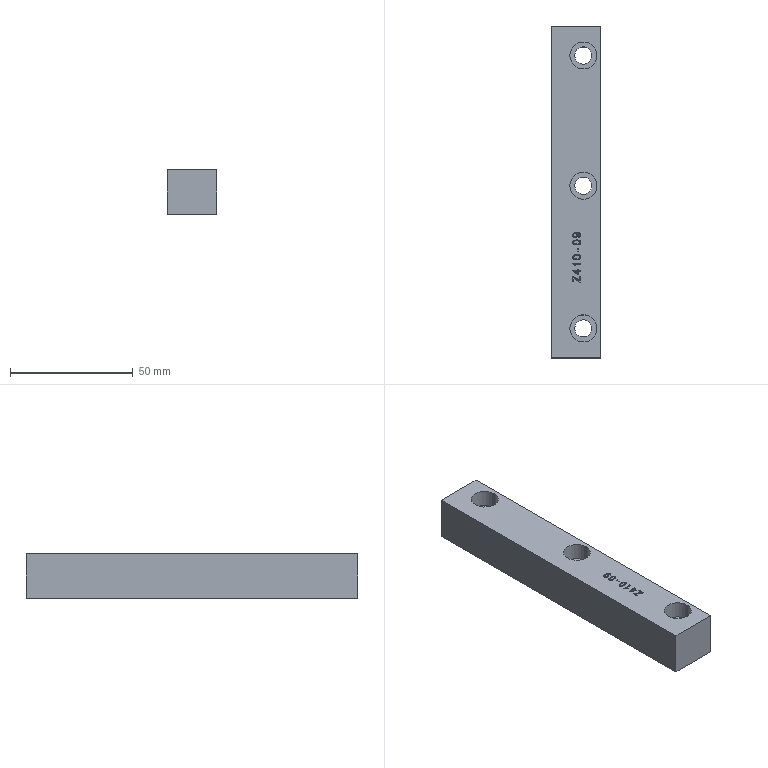Part | Creo | 1 solid | 141 faces | box 20 x 135 x 18 mm | volume 45331 mm3 | other 79 | plane 49 | cylinder 13 | commonest cylinder face diameters 7 x6 11 x6 45.582 x1